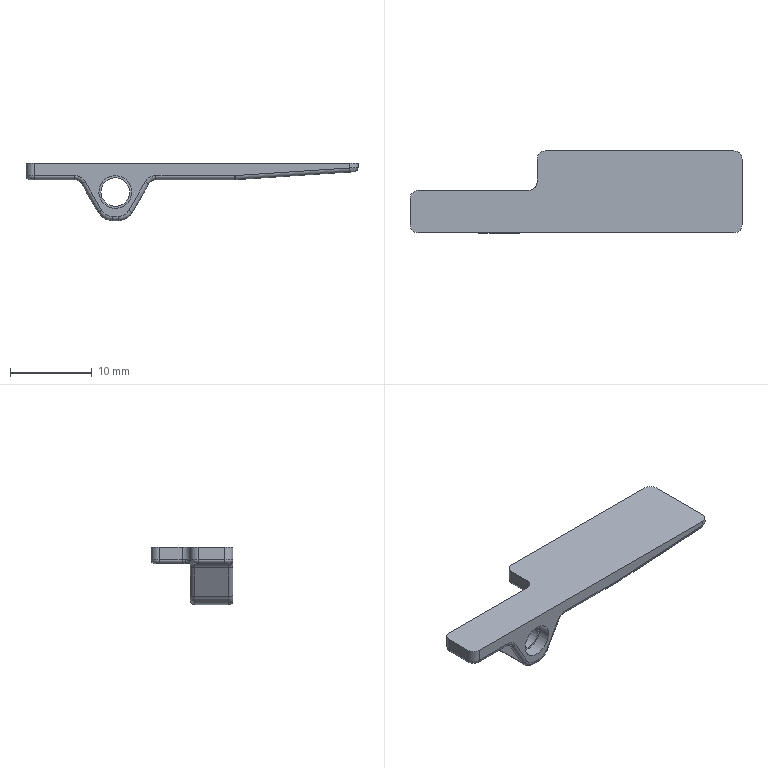CAM job | Mastercam | 3-axis milling, 5-axis milling | part box 40.5 x 10 x 7 mm | stock box 46 x 17 x 7 mm
Tools:
tool_number,name,type,diameter_mm,corner_radius_mm,flutes,flute_length_mm,overall_length_mm,shoulder_length_mm,holder_diameter_mm,length_offset,diameter_offset,default_rpm,default_feed_mm_min,default_plunge_mm_min,coolant
1,2 Ball Mill / Bull Nose Mill,ball end mill,2,1,4,4,100,4,50,1,1,8000,3000,600,COOL_OFF
2,2 Flat End Mill,end mill,2,0,4,25,75,25,50,2,2,5000,600,600,COOL_OFF
3,3 Flat End Mill,end mill,3,0,4,25,75,25,50,3,3,6000,1500,600,COOL_OFF
6,6 Flat End Mill,end mill,6,0,4,25,75,25,50,6,6,7000,3000,600,COOL_OFF
7,4 Chamfer Mill,chamfer mill,4,0,4,25,75,30,50,7,7,6500,1000,600,COOL_OFF
10,10 Flat End Mill,end mill,10,0,4,25,75,25,50,10,10,6500,1000,600,COOL_OFF
20,63 Flat End Mill,end mill,63,0,4,25,75,25,50,20,20,4000,2000,600,COOL_OFF
Operations:
seq,operation,operation_type,tool_number,tool_name,tool_diameter_mm,spindle_rpm,feed_mm_min,plunge_mm_min,retract_mm_min,cycle_time_s,wcs,posted,nc_file
1,Contour (2D) - [WCS: Plane] - [Tplane: Plane],Contour,10,10 Flat End Mill,10,6500,1000,600,1200,9.342,Plane,yes,.nc
2,Contour (Remachining) - [WCS: Plane] - [Tplane: Plane],Contour,2,2 Flat End Mill,2,5000,600,600,1200,2.208,Plane,yes,.nc
3,Facing - [WCS: Plane-1] - [Tplane: Plane-1],Facing,20,63 Flat End Mill,63,4000,2000,600,1200,73.707,Plane-1,yes,.nc
4,Contour (2D chamfer) - [WCS: Plane-1] - [Tplane: Plane-1],Contour,7,4 Chamfer Mill,4,6500,1000,600,1200,6.922,Plane-1,yes,.nc
5,3D High Speed (Waterline) - [WCS: Plane-2] - [Tplane: Plane-2],HighSpeed3D,3,3 Flat End Mill,3,6000,1000,600,1200,3.191,Plane-2,yes,.nc
6,Contour (2D) - [WCS: Plane-2] - [Tplane: Plane-2],Contour,3,3 Flat End Mill,3,6000,500,600,1200,1.159,Plane-2,yes,.nc
7,Contour (Ramp) - [WCS: Plane-2] - [Tplane: Plane-2],Contour,3,3 Flat End Mill,3,6000,500,600,1200,1.589,Plane-2,yes,.nc
8,Contour (2D chamfer) - [WCS: Plane-2] - [Tplane: Plane-2],Contour,7,4 Chamfer Mill,4,6500,1000,600,1200,1.285,Plane-2,yes,.nc
9,2D High Speed (2D Area Mill) - [WCS: Plane-3] - [Tplane: Plane-1],HighSpeed2D,3,3 Flat End Mill,3,7000,3000,600,1200,25.649,Plane-3,yes,.nc
10,Contour (2D) - [WCS: Plane-3] - [Tplane: Plane-1],Contour,3,3 Flat End Mill,3,6000,500,600,1200,12.127,Plane-3,yes,.nc
11,Contour (2D chamfer) - [WCS: Plane-3] - [Tplane: Plane-1],Contour,7,4 Chamfer Mill,4,6500,1000,600,1200,6.719,Plane-3,yes,.nc
12,3D High Speed (Area roughing) - [WCS: Plane-1] - [Tplane: Plane-1],HighSpeed3D,6,6 Flat End Mill,6,7000,2000,600,1200,117.743,Plane-1,yes,.nc
13,Surface Finish Flowline - [WCS: Plane-1] - [Tplane: Plane-1],MultiSurfaceFinishFlowline,1,2 Ball Mill / Bull Nose Mill,2,8000,2000,600,1200,125.308,Plane-1,yes,.nc
14,Unified Morph - [WCS: Plane-1] - [Tplane: Plane-1],461,1,2 Ball Mill / Bull Nose Mill,2,8000,800,600,1200,136.453,Plane-1,yes,.nc